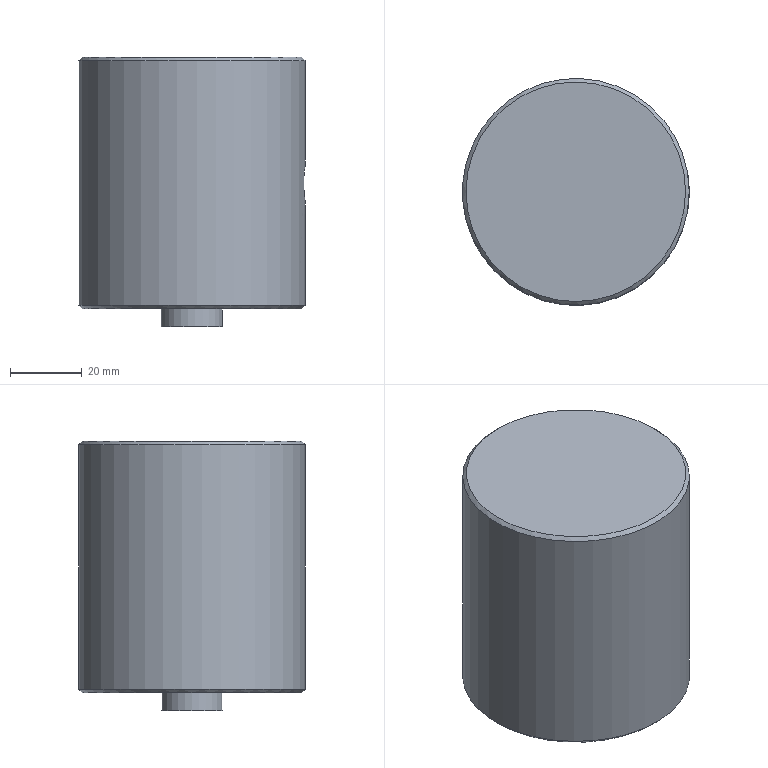Part | NX | features solid 2 | 1 solid | 11 faces | box 63 x 63 x 75 mm | volume 218186 mm3 | plane 5 | cylinder 4 | cone 2 | commonest cylinder face diameters 6 x1 10 x1 17 x1 63 x1
STEP:
#1=CARTESIAN_POINT('',(1366.5,1000.,-134.));
#2=VERTEX_POINT('',#1);
#3=CARTESIAN_POINT('',(1335.,1000.,-134.));
#4=DIRECTION('',(0.,0.,1.));
#5=DIRECTION('',(1.,0.,0.));
#6=AXIS2_PLACEMENT_3D('',#3,#4,#5);
#7=CIRCLE('',#6,31.5);
#8=EDGE_CURVE('',#2,#2,#7,.T.);
#9=ORIENTED_EDGE('',*,*,#8,.T.);
#10=EDGE_LOOP('',(#9));
#11=FACE_BOUND('',#10,.T.);
#12=CARTESIAN_POINT('',(1366.5,1000.,-66.));
#13=VERTEX_POINT('',#12);
#14=CARTESIAN_POINT('',(1335.,1000.,-66.));
#15=DIRECTION('',(0.,0.,1.));
#16=DIRECTION('',(1.,0.,0.));
#17=AXIS2_PLACEMENT_3D('',#14,#15,#16);
#18=CIRCLE('',#17,31.5);
#19=EDGE_CURVE('',#13,#13,#18,.F.);
#20=ORIENTED_EDGE('',*,*,#19,.T.);
#21=EDGE_LOOP('',(#20));
#22=FACE_BOUND('',#21,.T.);
#23=CARTESIAN_POINT('',(1366.112,1004.93,-99.165));
#24=VERTEX_POINT('',#23);
#25=CARTESIAN_POINT('',(1366.4,1003.208,-95.482));
#26=CARTESIAN_POINT('',(1366.017,1005.465,-99.074));
#27=CARTESIAN_POINT('',(1366.203,1004.513,-103.213));
#28=CARTESIAN_POINT('',(1366.583,1000.931,-105.462));
#29=CARTESIAN_POINT('',(1366.4,996.788,-104.516));
#30=CARTESIAN_POINT('',(1366.017,994.538,-100.927));
#31=CARTESIAN_POINT('',(1366.203,995.482,-96.793));
#32=CARTESIAN_POINT('',(1366.583,999.07,-94.538));
#33=CARTESIAN_POINT('',(1366.4,1003.208,-95.482));
#34=CARTESIAN_POINT('',(1366.017,1005.465,-99.074));
#35=CARTESIAN_POINT('',(1366.203,1004.513,-103.213));
#36=B_SPLINE_CURVE_WITH_KNOTS('',3,(#25,#26,#27,#28,#29,#30,#31,#32,#33,#34,#35),.UNSPECIFIED.,.T.,.F.,(1,1,1,1,1,1,1,1,1,1,1,1,1,1,1),(-0.01174,-0.007828,-0.003914,0.,0.003914,0.007828,0.01174,0.01566,0.01957,0.02348,0.0274,0.03131,0.03523,0.03914,0.04305),.UNSPECIFIED.);
#37=EDGE_CURVE('',#24,#24,#36,.T.);
#38=ORIENTED_EDGE('',*,*,#37,.T.);
#39=EDGE_LOOP('',(#38));
#40=FACE_BOUND('',#39,.T.);
#41=CARTESIAN_POINT('',(1335.,1000.,-90.));
#42=DIRECTION('',(0.,0.,-1.));
#43=DIRECTION('',(-1.,0.,0.));
#44=AXIS2_PLACEMENT_3D('',#41,#42,#43);
#45=CYLINDRICAL_SURFACE('',#44,31.5);
#46=ADVANCED_FACE('',(#11,#22,#40),#45,.T.);
#47=CARTESIAN_POINT('',(1365.5,1000.,-65.));
#48=VERTEX_POINT('',#47);
#49=CARTESIAN_POINT('',(1335.,1000.,-65.));
#50=DIRECTION('',(0.,0.,1.));
#51=DIRECTION('',(1.,0.,0.));
#52=AXIS2_PLACEMENT_3D('',#49,#50,#51);
#53=CIRCLE('',#52,30.5);
#54=EDGE_CURVE('',#48,#48,#53,.T.);
#55=ORIENTED_EDGE('',*,*,#54,.T.);
#56=EDGE_LOOP('',(#55));
#57=FACE_BOUND('',#56,.T.);
#58=CARTESIAN_POINT('',(1335.,1000.,-65.));
#59=DIRECTION('',(0.,0.,1.));
#60=DIRECTION('',(1.,0.,0.));
#61=AXIS2_PLACEMENT_3D('',#58,#59,#60);
#62=PLANE('',#61);
#63=ADVANCED_FACE('',(#57),#62,.T.);
#64=CARTESIAN_POINT('',(1365.5,1000.,-135.));
#65=VERTEX_POINT('',#64);
#66=CARTESIAN_POINT('',(1335.,1000.,-135.));
#67=DIRECTION('',(0.,0.,1.));
#68=DIRECTION('',(1.,0.,0.));
#69=AXIS2_PLACEMENT_3D('',#66,#67,#68);
#70=CIRCLE('',#69,30.5);
#71=EDGE_CURVE('',#65,#65,#70,.F.);
#72=ORIENTED_EDGE('',*,*,#71,.T.);
#73=EDGE_LOOP('',(#72));
#74=FACE_BOUND('',#73,.T.);
#75=CARTESIAN_POINT('',(1343.5,1000.,-135.));
#76=VERTEX_POINT('',#75);
#77=CARTESIAN_POINT('',(1335.,1000.,-135.));
#78=DIRECTION('',(0.,0.,1.));
#79=DIRECTION('',(1.,0.,0.));
#80=AXIS2_PLACEMENT_3D('',#77,#78,#79);
#81=CIRCLE('',#80,8.5);
#82=EDGE_CURVE('',#76,#76,#81,.T.);
#83=ORIENTED_EDGE('',*,*,#82,.T.);
#84=EDGE_LOOP('',(#83));
#85=FACE_BOUND('',#84,.T.);
#86=CARTESIAN_POINT('',(1335.,1000.,-135.));
#87=DIRECTION('',(0.,0.,1.));
#88=DIRECTION('',(1.,0.,0.));
#89=AXIS2_PLACEMENT_3D('',#86,#87,#88);
#90=PLANE('',#89);
#91=ADVANCED_FACE('',(#74,#85),#90,.F.);
#92=CARTESIAN_POINT('',(1343.5,1000.,-140.));
#93=VERTEX_POINT('',#92);
#94=CARTESIAN_POINT('',(1335.,1000.,-140.));
#95=DIRECTION('',(0.,0.,1.));
#96=DIRECTION('',(1.,0.,0.));
#97=AXIS2_PLACEMENT_3D('',#94,#95,#96);
#98=CIRCLE('',#97,8.5);
#99=EDGE_CURVE('',#93,#93,#98,.T.);
#100=ORIENTED_EDGE('',*,*,#99,.T.);
#101=EDGE_LOOP('',(#100));
#102=FACE_BOUND('',#101,.T.);
#103=ORIENTED_EDGE('',*,*,#82,.F.);
#104=EDGE_LOOP('',(#103));
#105=FACE_BOUND('',#104,.T.);
#106=CARTESIAN_POINT('',(1335.,1000.,-125.));
#107=DIRECTION('',(0.,0.,1.));
#108=DIRECTION('',(1.,0.,0.));
#109=AXIS2_PLACEMENT_3D('',#106,#107,#108);
#110=CYLINDRICAL_SURFACE('',#109,8.5);
#111=ADVANCED_FACE('',(#102,#105),#110,.T.);
#112=ORIENTED_EDGE('',*,*,#99,.F.);
#113=EDGE_LOOP('',(#112));
#114=FACE_BOUND('',#113,.T.);
#115=CARTESIAN_POINT('',(1335.,1000.,-140.));
#116=DIRECTION('',(0.,0.,1.));
#117=DIRECTION('',(1.,0.,0.));
#118=AXIS2_PLACEMENT_3D('',#115,#116,#117);
#119=PLANE('',#118);
#120=ADVANCED_FACE('',(#114),#119,.F.);
#121=CARTESIAN_POINT('',(1365.5,1000.,-105.));
#122=VERTEX_POINT('',#121);
#123=CARTESIAN_POINT('',(1365.5,1000.,-100.));
#124=DIRECTION('',(1.,0.,0.));
#125=DIRECTION('',(0.,0.,-1.));
#126=AXIS2_PLACEMENT_3D('',#123,#124,#125);
#127=CIRCLE('',#126,5.);
#128=EDGE_CURVE('',#122,#122,#127,.T.);
#129=ORIENTED_EDGE('',*,*,#128,.F.);
#130=EDGE_LOOP('',(#129));
#131=FACE_BOUND('',#130,.T.);
#132=ORIENTED_EDGE('',*,*,#37,.F.);
#133=EDGE_LOOP('',(#132));
#134=FACE_BOUND('',#133,.T.);
#135=CARTESIAN_POINT('',(1354.,1000.,-100.));
#136=DIRECTION('',(1.,0.,0.));
#137=DIRECTION('',(0.,0.,-1.));
#138=AXIS2_PLACEMENT_3D('',#135,#136,#137);
#139=CYLINDRICAL_SURFACE('',#138,5.);
#140=ADVANCED_FACE('',(#131,#134),#139,.F.);
#141=CARTESIAN_POINT('',(1365.5,1000.,-103.));
#142=VERTEX_POINT('',#141);
#143=CARTESIAN_POINT('',(1365.5,1000.,-100.));
#144=DIRECTION('',(1.,0.,0.));
#145=DIRECTION('',(0.,0.,-1.));
#146=AXIS2_PLACEMENT_3D('',#143,#144,#145);
#147=CIRCLE('',#146,3.);
#148=EDGE_CURVE('',#142,#142,#147,.F.);
#149=ORIENTED_EDGE('',*,*,#148,.T.);
#150=EDGE_LOOP('',(#149));
#151=FACE_BOUND('',#150,.T.);
#152=ORIENTED_EDGE('',*,*,#128,.T.);
#153=EDGE_LOOP('',(#152));
#154=FACE_BOUND('',#153,.T.);
#155=CARTESIAN_POINT('',(1365.5,1000.,-100.));
#156=DIRECTION('',(1.,0.,0.));
#157=DIRECTION('',(0.,0.,-1.));
#158=AXIS2_PLACEMENT_3D('',#155,#156,#157);
#159=PLANE('',#158);
#160=ADVANCED_FACE('',(#151,#154),#159,.T.);
#161=CARTESIAN_POINT('',(1334.,1000.,-97.));
#162=VERTEX_POINT('',#161);
#163=CARTESIAN_POINT('',(1334.,1000.,-100.));
#164=DIRECTION('',(-1.,0.,0.));
#165=DIRECTION('',(0.,0.,1.));
#166=AXIS2_PLACEMENT_3D('',#163,#164,#165);
#167=CIRCLE('',#166,3.);
#168=EDGE_CURVE('',#162,#162,#167,.T.);
#169=ORIENTED_EDGE('',*,*,#168,.F.);
#170=EDGE_LOOP('',(#169));
#171=FACE_BOUND('',#170,.T.);
#172=CARTESIAN_POINT('',(1334.,1000.,-105.));
#173=DIRECTION('',(-1.,0.,0.));
#174=DIRECTION('',(0.,0.,1.));
#175=AXIS2_PLACEMENT_3D('',#172,#173,#174);
#176=PLANE('',#175);
#177=ADVANCED_FACE('',(#171),#176,.F.);
#178=ORIENTED_EDGE('',*,*,#168,.T.);
#179=EDGE_LOOP('',(#178));
#180=FACE_BOUND('',#179,.T.);
#181=ORIENTED_EDGE('',*,*,#148,.F.);
#182=EDGE_LOOP('',(#181));
#183=FACE_BOUND('',#182,.T.);
#184=CARTESIAN_POINT('',(1354.,1000.,-100.));
#185=DIRECTION('',(-1.,0.,0.));
#186=DIRECTION('',(0.,0.,1.));
#187=AXIS2_PLACEMENT_3D('',#184,#185,#186);
#188=CYLINDRICAL_SURFACE('',#187,3.);
#189=ADVANCED_FACE('',(#180,#183),#188,.F.);
#190=ORIENTED_EDGE('',*,*,#54,.F.);
#191=EDGE_LOOP('',(#190));
#192=FACE_BOUND('',#191,.T.);
#193=ORIENTED_EDGE('',*,*,#19,.F.);
#194=EDGE_LOOP('',(#193));
#195=FACE_BOUND('',#194,.T.);
#196=CARTESIAN_POINT('',(1335.,1000.,-66.));
#197=DIRECTION('',(0.,0.,-1.));
#198=DIRECTION('',(-1.,0.,0.));
#199=AXIS2_PLACEMENT_3D('',#196,#197,#198);
#200=CONICAL_SURFACE('',#199,31.5,0.7854);
#201=ADVANCED_FACE('',(#192,#195),#200,.T.);
#202=ORIENTED_EDGE('',*,*,#71,.F.);
#203=EDGE_LOOP('',(#202));
#204=FACE_BOUND('',#203,.T.);
#205=ORIENTED_EDGE('',*,*,#8,.F.);
#206=EDGE_LOOP('',(#205));
#207=FACE_BOUND('',#206,.T.);
#208=CARTESIAN_POINT('',(1335.,1000.,-134.));
#209=DIRECTION('',(0.,0.,1.));
#210=DIRECTION('',(1.,0.,0.));
#211=AXIS2_PLACEMENT_3D('',#208,#209,#210);
#212=CONICAL_SURFACE('',#211,31.5,0.7854);
#213=ADVANCED_FACE('',(#204,#207),#212,.T.);
#214=CLOSED_SHELL('',(#46,#63,#91,#111,#120,#140,#160,#177,#189,#201,#213));
#215=MANIFOLD_SOLID_BREP('',#214);
#216=(LENGTH_UNIT()NAMED_UNIT(*)SI_UNIT(.MILLI.,.METRE.));
#217=UNCERTAINTY_MEASURE_WITH_UNIT(LENGTH_MEASURE(0.0508),#216,'','');
#218=(NAMED_UNIT(*)PLANE_ANGLE_UNIT()SI_UNIT($,.RADIAN.));
#219=(NAMED_UNIT(*)SI_UNIT($,.STERADIAN.)SOLID_ANGLE_UNIT());
#220=(GEOMETRIC_REPRESENTATION_CONTEXT(3)GLOBAL_UNCERTAINTY_ASSIGNED_CONTEXT((#217))GLOBAL_UNIT_ASSIGNED_CONTEXT((#216,#218,#219))REPRESENTATION_CONTEXT('',''));
#221=ADVANCED_BREP_SHAPE_REPRESENTATION('',(#215),#220);